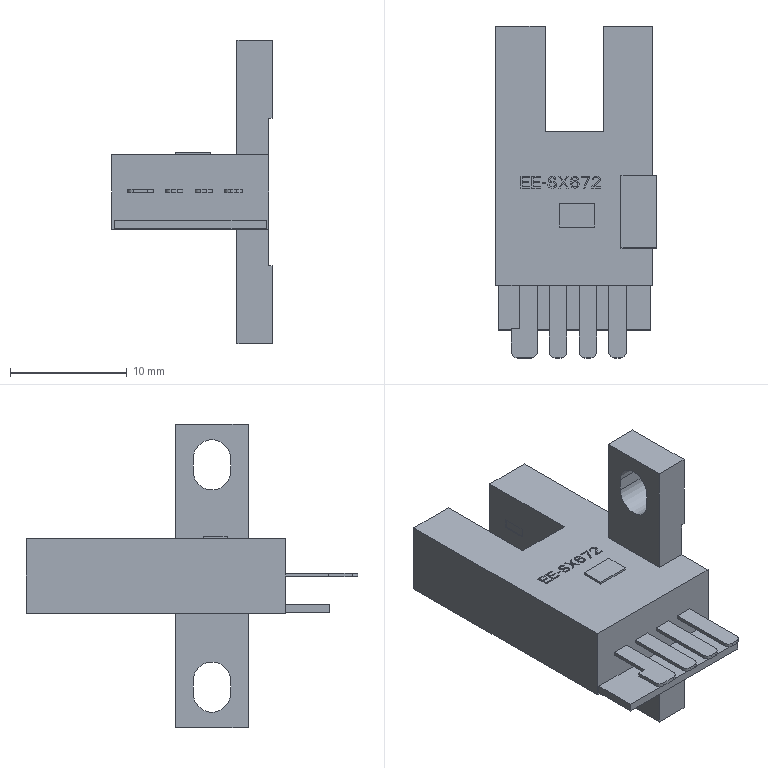Part | NX | 1 solid | 278 faces | box 13.7 x 28.4 x 26 mm | volume 1946 mm3 | plane 266 | cylinder 12 | commonest cylinder face diameters 1 x8 3.2 x4